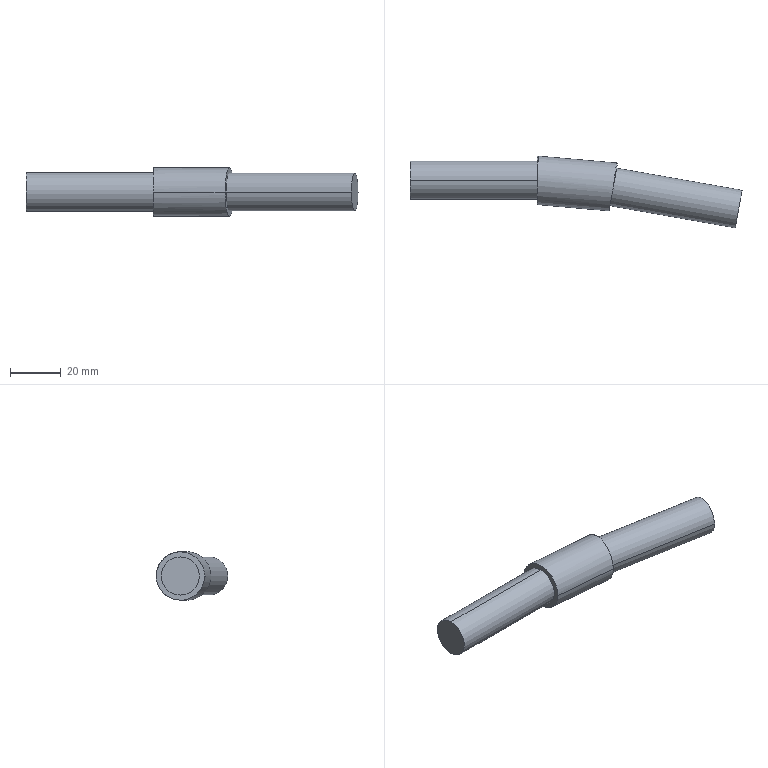Part | SolidWorks | features ICE 2, Sweep 1 | 1 solid | 13 faces | box 130.429 x 28.183 x 19 mm | volume 26177 mm3 | cylinder 9 | plane 4 | commonest cylinder face diameters 19 x5 15 x4
STEP:
#1=CARTESIAN_POINT('',(81.188,4.771,0.));
#2=VERTEX_POINT('',#1);
#3=CARTESIAN_POINT('',(78.583,-10.001,0.));
#4=VERTEX_POINT('',#3);
#5=CARTESIAN_POINT('',(79.886,-2.615,0.));
#6=DIRECTION('',(0.9848,-0.1736,0.));
#7=DIRECTION('',(0.1736,0.9848,0.));
#8=AXIS2_PLACEMENT_3D('',#5,#6,#7);
#9=CIRCLE('',#8,7.5);
#10=EDGE_CURVE('',#2,#4,#9,.T.);
#11=ORIENTED_EDGE('',*,*,#10,.T.);
#12=CARTESIAN_POINT('',(127.824,-18.683,0.));
#13=VERTEX_POINT('',#12);
#14=CARTESIAN_POINT('',(78.583,-10.001,0.));
#15=DIRECTION('',(0.9848,-0.1736,0.));
#16=VECTOR('',#15,1000.);
#17=LINE('',#14,#16);
#18=EDGE_CURVE('',#4,#13,#17,.T.);
#19=ORIENTED_EDGE('',*,*,#18,.T.);
#20=CARTESIAN_POINT('',(130.429,-3.911,0.));
#21=VERTEX_POINT('',#20);
#22=CARTESIAN_POINT('',(129.126,-11.297,0.));
#23=DIRECTION('',(0.9848,-0.1736,0.));
#24=DIRECTION('',(0.1736,0.9848,0.));
#25=AXIS2_PLACEMENT_3D('',#22,#23,#24);
#26=CIRCLE('',#25,7.5);
#27=EDGE_CURVE('',#21,#13,#26,.T.);
#28=ORIENTED_EDGE('',*,*,#27,.F.);
#29=CARTESIAN_POINT('',(81.188,4.771,0.));
#30=DIRECTION('',(0.9848,-0.1736,0.));
#31=VECTOR('',#30,1000.);
#32=LINE('',#29,#31);
#33=EDGE_CURVE('',#2,#21,#32,.T.);
#34=ORIENTED_EDGE('',*,*,#33,.F.);
#35=EDGE_LOOP('',(#11,#19,#28,#34));
#36=FACE_OUTER_BOUND('',#35,.T.);
#37=CARTESIAN_POINT('',(79.886,-2.615,0.));
#38=DIRECTION('',(0.9848,-0.1736,0.));
#39=DIRECTION('',(0.1736,0.9848,0.));
#40=AXIS2_PLACEMENT_3D('',#37,#38,#39);
#41=CYLINDRICAL_SURFACE('',#40,7.5);
#42=ADVANCED_FACE('',(#36),#41,.T.);
#43=CARTESIAN_POINT('',(50.,0.,7.5));
#44=VERTEX_POINT('',#43);
#45=CARTESIAN_POINT('',(50.,0.,-7.5));
#46=VERTEX_POINT('',#45);
#47=CARTESIAN_POINT('',(50.,0.,0.));
#48=DIRECTION('',(-1.,0.,0.));
#49=DIRECTION('',(0.,0.,1.));
#50=AXIS2_PLACEMENT_3D('',#47,#48,#49);
#51=CIRCLE('',#50,7.5);
#52=EDGE_CURVE('',#44,#46,#51,.T.);
#53=ORIENTED_EDGE('',*,*,#52,.T.);
#54=CARTESIAN_POINT('',(0.,0.,-7.5));
#55=VERTEX_POINT('',#54);
#56=CARTESIAN_POINT('',(50.,0.,-7.5));
#57=DIRECTION('',(-1.,0.,0.));
#58=VECTOR('',#57,1000.);
#59=LINE('',#56,#58);
#60=EDGE_CURVE('',#46,#55,#59,.T.);
#61=ORIENTED_EDGE('',*,*,#60,.T.);
#62=CARTESIAN_POINT('',(0.,0.,7.5));
#63=VERTEX_POINT('',#62);
#64=CARTESIAN_POINT('',(0.,0.,0.));
#65=DIRECTION('',(-1.,0.,0.));
#66=DIRECTION('',(0.,0.,1.));
#67=AXIS2_PLACEMENT_3D('',#64,#65,#66);
#68=CIRCLE('',#67,7.5);
#69=EDGE_CURVE('',#63,#55,#68,.T.);
#70=ORIENTED_EDGE('',*,*,#69,.F.);
#71=CARTESIAN_POINT('',(50.,0.,7.5));
#72=DIRECTION('',(-1.,0.,0.));
#73=VECTOR('',#72,1000.);
#74=LINE('',#71,#73);
#75=EDGE_CURVE('',#44,#63,#74,.T.);
#76=ORIENTED_EDGE('',*,*,#75,.F.);
#77=EDGE_LOOP('',(#53,#61,#70,#76));
#78=FACE_OUTER_BOUND('',#77,.T.);
#79=CARTESIAN_POINT('',(50.,0.,0.));
#80=DIRECTION('',(-1.,0.,0.));
#81=DIRECTION('',(0.,0.,1.));
#82=AXIS2_PLACEMENT_3D('',#79,#80,#81);
#83=CYLINDRICAL_SURFACE('',#82,7.5);
#84=ADVANCED_FACE('',(#78),#83,.T.);
#85=CARTESIAN_POINT('',(81.127,6.813,0.));
#86=VERTEX_POINT('',#85);
#87=CARTESIAN_POINT('',(79.886,-2.615,-9.5));
#88=VERTEX_POINT('',#87);
#89=CARTESIAN_POINT('',(81.127,6.813,0.));
#90=CARTESIAN_POINT('',(81.127,6.813,-5.565));
#91=CARTESIAN_POINT('',(80.613,2.908,-9.5));
#92=CARTESIAN_POINT('',(79.886,-2.615,-9.5));
#93=(BOUNDED_CURVE()B_SPLINE_CURVE(3,(#89,#90,#91,#92),.UNSPECIFIED.,.F.,.T.)B_SPLINE_CURVE_WITH_KNOTS((4,4),(0.,1.571),.UNSPECIFIED.)CURVE()GEOMETRIC_REPRESENTATION_ITEM()RATIONAL_B_SPLINE_CURVE((1.,0.8047,0.8047,1.))REPRESENTATION_ITEM(''));
#94=EDGE_CURVE('',#86,#88,#93,.T.);
#95=ORIENTED_EDGE('',*,*,#94,.F.);
#96=CARTESIAN_POINT('',(81.535,6.741,0.));
#97=VERTEX_POINT('',#96);
#98=CARTESIAN_POINT('',(81.535,6.741,0.));
#99=DIRECTION('',(0.9848,-0.1736,0.));
#100=VECTOR('',#99,1000.);
#101=LINE('',#98,#100);
#102=EDGE_CURVE('',#86,#97,#101,.T.);
#103=ORIENTED_EDGE('',*,*,#102,.T.);
#104=CARTESIAN_POINT('',(79.886,-2.615,0.));
#105=DIRECTION('',(0.9848,-0.1736,0.));
#106=DIRECTION('',(0.1736,0.9848,0.));
#107=AXIS2_PLACEMENT_3D('',#104,#105,#106);
#108=CIRCLE('',#107,9.5);
#109=EDGE_CURVE('',#88,#97,#108,.T.);
#110=ORIENTED_EDGE('',*,*,#109,.F.);
#111=EDGE_LOOP('',(#95,#103,#110));
#112=FACE_OUTER_BOUND('',#111,.T.);
#113=CARTESIAN_POINT('',(79.886,-2.615,0.));
#114=DIRECTION('',(0.9848,-0.1736,0.));
#115=DIRECTION('',(0.1736,0.9848,0.));
#116=AXIS2_PLACEMENT_3D('',#113,#114,#115);
#117=CYLINDRICAL_SURFACE('',#116,9.5);
#118=ADVANCED_FACE('',(#112),#117,.T.);
#119=CARTESIAN_POINT('',(50.,0.,9.5));
#120=VERTEX_POINT('',#119);
#121=CARTESIAN_POINT('',(50.,-9.536,0.));
#122=VERTEX_POINT('',#121);
#123=CARTESIAN_POINT('',(50.,0.,9.5));
#124=CARTESIAN_POINT('',(50.,-5.586,9.5));
#125=CARTESIAN_POINT('',(50.,-9.536,5.565));
#126=CARTESIAN_POINT('',(50.,-9.536,0.));
#127=(BOUNDED_CURVE()B_SPLINE_CURVE(3,(#123,#124,#125,#126),.UNSPECIFIED.,.F.,.T.)B_SPLINE_CURVE_WITH_KNOTS((4,4),(4.712,6.283),.UNSPECIFIED.)CURVE()GEOMETRIC_REPRESENTATION_ITEM()RATIONAL_B_SPLINE_CURVE((1.,0.8047,0.8047,1.))REPRESENTATION_ITEM(''));
#128=EDGE_CURVE('',#120,#122,#127,.T.);
#129=ORIENTED_EDGE('',*,*,#128,.T.);
#130=CARTESIAN_POINT('',(78.23,-12.006,0.));
#131=VERTEX_POINT('',#130);
#132=CARTESIAN_POINT('',(49.172,-9.464,0.));
#133=DIRECTION('',(0.9962,-0.08716,0.));
#134=VECTOR('',#133,1000.);
#135=LINE('',#132,#134);
#136=EDGE_CURVE('',#122,#131,#135,.T.);
#137=ORIENTED_EDGE('',*,*,#136,.T.);
#138=CARTESIAN_POINT('',(79.886,-2.615,9.5));
#139=VERTEX_POINT('',#138);
#140=CARTESIAN_POINT('',(78.23,-12.006,0.));
#141=CARTESIAN_POINT('',(78.23,-12.006,5.565));
#142=CARTESIAN_POINT('',(78.916,-8.116,9.5));
#143=CARTESIAN_POINT('',(79.886,-2.615,9.5));
#144=(BOUNDED_CURVE()B_SPLINE_CURVE(3,(#140,#141,#142,#143),.UNSPECIFIED.,.F.,.T.)B_SPLINE_CURVE_WITH_KNOTS((4,4),(3.142,4.712),.UNSPECIFIED.)CURVE()GEOMETRIC_REPRESENTATION_ITEM()RATIONAL_B_SPLINE_CURVE((1.,0.8047,0.8047,1.))REPRESENTATION_ITEM(''));
#145=EDGE_CURVE('',#131,#139,#144,.T.);
#146=ORIENTED_EDGE('',*,*,#145,.T.);
#147=CARTESIAN_POINT('',(79.886,-2.615,9.5));
#148=CARTESIAN_POINT('',(80.613,2.908,9.5));
#149=CARTESIAN_POINT('',(81.127,6.813,5.565));
#150=CARTESIAN_POINT('',(81.127,6.813,0.));
#151=(BOUNDED_CURVE()B_SPLINE_CURVE(3,(#147,#148,#149,#150),.UNSPECIFIED.,.F.,.T.)B_SPLINE_CURVE_WITH_KNOTS((4,4),(4.712,6.283),.UNSPECIFIED.)CURVE()GEOMETRIC_REPRESENTATION_ITEM()RATIONAL_B_SPLINE_CURVE((1.,0.8047,0.8047,1.))REPRESENTATION_ITEM(''));
#152=EDGE_CURVE('',#139,#86,#151,.T.);
#153=ORIENTED_EDGE('',*,*,#152,.T.);
#154=CARTESIAN_POINT('',(50.415,9.5,0.));
#155=VERTEX_POINT('',#154);
#156=CARTESIAN_POINT('',(50.828,9.464,0.));
#157=DIRECTION('',(0.9962,-0.08716,0.));
#158=VECTOR('',#157,1000.);
#159=LINE('',#156,#158);
#160=EDGE_CURVE('',#155,#86,#159,.T.);
#161=ORIENTED_EDGE('',*,*,#160,.F.);
#162=CARTESIAN_POINT('',(50.415,9.5,0.));
#163=CARTESIAN_POINT('',(50.415,9.5,5.565));
#164=CARTESIAN_POINT('',(50.243,5.565,9.5));
#165=CARTESIAN_POINT('',(50.,0.,9.5));
#166=(BOUNDED_CURVE()B_SPLINE_CURVE(3,(#162,#163,#164,#165),.UNSPECIFIED.,.F.,.T.)B_SPLINE_CURVE_WITH_KNOTS((4,4),(3.142,4.712),.UNSPECIFIED.)CURVE()GEOMETRIC_REPRESENTATION_ITEM()RATIONAL_B_SPLINE_CURVE((1.,0.8047,0.8047,1.))REPRESENTATION_ITEM(''));
#167=EDGE_CURVE('',#155,#120,#166,.T.);
#168=ORIENTED_EDGE('',*,*,#167,.T.);
#169=EDGE_LOOP('',(#129,#137,#146,#153,#161,#168));
#170=FACE_OUTER_BOUND('',#169,.T.);
#171=CARTESIAN_POINT('',(50.,0.,0.));
#172=DIRECTION('',(0.9962,-0.08716,0.));
#173=DIRECTION('',(0.08716,0.9962,0.));
#174=AXIS2_PLACEMENT_3D('',#171,#172,#173);
#175=CYLINDRICAL_SURFACE('',#174,9.5);
#176=ADVANCED_FACE('',(#170),#175,.T.);
#177=ORIENTED_EDGE('',*,*,#136,.F.);
#178=CARTESIAN_POINT('',(50.,0.,-9.5));
#179=VERTEX_POINT('',#178);
#180=CARTESIAN_POINT('',(50.,-9.536,0.));
#181=CARTESIAN_POINT('',(50.,-9.536,-5.565));
#182=CARTESIAN_POINT('',(50.,-5.586,-9.5));
#183=CARTESIAN_POINT('',(50.,0.,-9.5));
#184=(BOUNDED_CURVE()B_SPLINE_CURVE(3,(#180,#181,#182,#183),.UNSPECIFIED.,.F.,.T.)B_SPLINE_CURVE_WITH_KNOTS((4,4),(0.,1.571),.UNSPECIFIED.)CURVE()GEOMETRIC_REPRESENTATION_ITEM()RATIONAL_B_SPLINE_CURVE((1.,0.8047,0.8047,1.))REPRESENTATION_ITEM(''));
#185=EDGE_CURVE('',#122,#179,#184,.T.);
#186=ORIENTED_EDGE('',*,*,#185,.T.);
#187=CARTESIAN_POINT('',(50.,0.,-9.5));
#188=CARTESIAN_POINT('',(50.243,5.565,-9.5));
#189=CARTESIAN_POINT('',(50.415,9.5,-5.565));
#190=CARTESIAN_POINT('',(50.415,9.5,0.));
#191=(BOUNDED_CURVE()B_SPLINE_CURVE(3,(#187,#188,#189,#190),.UNSPECIFIED.,.F.,.T.)B_SPLINE_CURVE_WITH_KNOTS((4,4),(1.571,3.142),.UNSPECIFIED.)CURVE()GEOMETRIC_REPRESENTATION_ITEM()RATIONAL_B_SPLINE_CURVE((1.,0.8047,0.8047,1.))REPRESENTATION_ITEM(''));
#192=EDGE_CURVE('',#179,#155,#191,.T.);
#193=ORIENTED_EDGE('',*,*,#192,.T.);
#194=ORIENTED_EDGE('',*,*,#160,.T.);
#195=ORIENTED_EDGE('',*,*,#94,.T.);
#196=CARTESIAN_POINT('',(79.886,-2.615,-9.5));
#197=CARTESIAN_POINT('',(78.916,-8.116,-9.5));
#198=CARTESIAN_POINT('',(78.23,-12.006,-5.565));
#199=CARTESIAN_POINT('',(78.23,-12.006,0.));
#200=(BOUNDED_CURVE()B_SPLINE_CURVE(3,(#196,#197,#198,#199),.UNSPECIFIED.,.F.,.T.)B_SPLINE_CURVE_WITH_KNOTS((4,4),(1.571,3.142),.UNSPECIFIED.)CURVE()GEOMETRIC_REPRESENTATION_ITEM()RATIONAL_B_SPLINE_CURVE((1.,0.8047,0.8047,1.))REPRESENTATION_ITEM(''));
#201=EDGE_CURVE('',#88,#131,#200,.T.);
#202=ORIENTED_EDGE('',*,*,#201,.T.);
#203=EDGE_LOOP('',(#177,#186,#193,#194,#195,#202));
#204=FACE_OUTER_BOUND('',#203,.T.);
#205=CARTESIAN_POINT('',(50.,0.,0.));
#206=DIRECTION('',(0.9962,-0.08716,0.));
#207=DIRECTION('',(0.08716,0.9962,0.));
#208=AXIS2_PLACEMENT_3D('',#205,#206,#207);
#209=CYLINDRICAL_SURFACE('',#208,9.5);
#210=ADVANCED_FACE('',(#204),#209,.T.);
#211=ORIENTED_EDGE('',*,*,#102,.F.);
#212=ORIENTED_EDGE('',*,*,#152,.F.);
#213=CARTESIAN_POINT('',(79.886,-2.615,0.));
#214=DIRECTION('',(0.9848,-0.1736,0.));
#215=DIRECTION('',(0.1736,0.9848,0.));
#216=AXIS2_PLACEMENT_3D('',#213,#214,#215);
#217=CIRCLE('',#216,9.5);
#218=EDGE_CURVE('',#97,#139,#217,.T.);
#219=ORIENTED_EDGE('',*,*,#218,.F.);
#220=EDGE_LOOP('',(#211,#212,#219));
#221=FACE_OUTER_BOUND('',#220,.T.);
#222=CARTESIAN_POINT('',(79.886,-2.615,0.));
#223=DIRECTION('',(0.9848,-0.1736,0.));
#224=DIRECTION('',(0.1736,0.9848,0.));
#225=AXIS2_PLACEMENT_3D('',#222,#223,#224);
#226=CYLINDRICAL_SURFACE('',#225,9.5);
#227=ADVANCED_FACE('',(#221),#226,.T.);
#228=CARTESIAN_POINT('',(50.,0.,0.));
#229=DIRECTION('',(-1.,0.,0.));
#230=DIRECTION('',(0.,0.,1.));
#231=AXIS2_PLACEMENT_3D('',#228,#229,#230);
#232=CIRCLE('',#231,9.5);
#233=EDGE_CURVE('',#120,#179,#232,.T.);
#234=ORIENTED_EDGE('',*,*,#233,.F.);
#235=ORIENTED_EDGE('',*,*,#167,.F.);
#236=ORIENTED_EDGE('',*,*,#192,.F.);
#237=EDGE_LOOP('',(#234,#235,#236));
#238=FACE_OUTER_BOUND('',#237,.T.);
#239=CARTESIAN_POINT('',(76.87,0.,0.));
#240=DIRECTION('',(-1.,0.,0.));
#241=DIRECTION('',(0.,0.,1.));
#242=AXIS2_PLACEMENT_3D('',#239,#240,#241);
#243=CYLINDRICAL_SURFACE('',#242,9.5);
#244=ADVANCED_FACE('',(#238),#243,.T.);
#245=ORIENTED_EDGE('',*,*,#233,.T.);
#246=ORIENTED_EDGE('',*,*,#185,.F.);
#247=ORIENTED_EDGE('',*,*,#128,.F.);
#248=EDGE_LOOP('',(#245,#246,#247));
#249=FACE_OUTER_BOUND('',#248,.T.);
#250=ORIENTED_EDGE('',*,*,#52,.F.);
#251=CARTESIAN_POINT('',(50.,0.,0.));
#252=DIRECTION('',(-1.,0.,0.));
#253=DIRECTION('',(0.,0.,1.));
#254=AXIS2_PLACEMENT_3D('',#251,#252,#253);
#255=CIRCLE('',#254,7.5);
#256=EDGE_CURVE('',#46,#44,#255,.T.);
#257=ORIENTED_EDGE('',*,*,#256,.F.);
#258=EDGE_LOOP('',(#250,#257));
#259=FACE_BOUND('',#258,.T.);
#260=CARTESIAN_POINT('',(50.,-5.576,0.));
#261=DIRECTION('',(-1.,0.,0.));
#262=DIRECTION('',(0.,0.,1.));
#263=AXIS2_PLACEMENT_3D('',#260,#261,#262);
#264=PLANE('',#263);
#265=ADVANCED_FACE('',(#249,#259),#264,.T.);
#266=ORIENTED_EDGE('',*,*,#60,.F.);
#267=ORIENTED_EDGE('',*,*,#256,.T.);
#268=ORIENTED_EDGE('',*,*,#75,.T.);
#269=CARTESIAN_POINT('',(0.,0.,0.));
#270=DIRECTION('',(-1.,0.,0.));
#271=DIRECTION('',(0.,0.,1.));
#272=AXIS2_PLACEMENT_3D('',#269,#270,#271);
#273=CIRCLE('',#272,7.5);
#274=EDGE_CURVE('',#55,#63,#273,.T.);
#275=ORIENTED_EDGE('',*,*,#274,.F.);
#276=EDGE_LOOP('',(#266,#267,#268,#275));
#277=FACE_OUTER_BOUND('',#276,.T.);
#278=CARTESIAN_POINT('',(50.,0.,0.));
#279=DIRECTION('',(-1.,0.,0.));
#280=DIRECTION('',(0.,0.,1.));
#281=AXIS2_PLACEMENT_3D('',#278,#279,#280);
#282=CYLINDRICAL_SURFACE('',#281,7.5);
#283=ADVANCED_FACE('',(#277),#282,.T.);
#284=ORIENTED_EDGE('',*,*,#69,.T.);
#285=ORIENTED_EDGE('',*,*,#274,.T.);
#286=EDGE_LOOP('',(#284,#285));
#287=FACE_OUTER_BOUND('',#286,.T.);
#288=CARTESIAN_POINT('',(0.,0.,0.));
#289=DIRECTION('',(1.,0.,0.));
#290=DIRECTION('',(0.,0.,-1.));
#291=AXIS2_PLACEMENT_3D('',#288,#289,#290);
#292=PLANE('',#291);
#293=ADVANCED_FACE('',(#287),#292,.F.);
#294=ORIENTED_EDGE('',*,*,#109,.T.);
#295=ORIENTED_EDGE('',*,*,#218,.T.);
#296=ORIENTED_EDGE('',*,*,#145,.F.);
#297=ORIENTED_EDGE('',*,*,#201,.F.);
#298=EDGE_LOOP('',(#294,#295,#296,#297));
#299=FACE_OUTER_BOUND('',#298,.T.);
#300=ORIENTED_EDGE('',*,*,#10,.F.);
#301=CARTESIAN_POINT('',(79.886,-2.615,0.));
#302=DIRECTION('',(0.9848,-0.1736,0.));
#303=DIRECTION('',(0.1736,0.9848,0.));
#304=AXIS2_PLACEMENT_3D('',#301,#302,#303);
#305=CIRCLE('',#304,7.5);
#306=EDGE_CURVE('',#4,#2,#305,.T.);
#307=ORIENTED_EDGE('',*,*,#306,.F.);
#308=EDGE_LOOP('',(#300,#307));
#309=FACE_BOUND('',#308,.T.);
#310=CARTESIAN_POINT('',(78.942,-7.966,0.));
#311=DIRECTION('',(0.9848,-0.1736,0.));
#312=DIRECTION('',(0.1736,0.9848,0.));
#313=AXIS2_PLACEMENT_3D('',#310,#311,#312);
#314=PLANE('',#313);
#315=ADVANCED_FACE('',(#299,#309),#314,.T.);
#316=ORIENTED_EDGE('',*,*,#18,.F.);
#317=ORIENTED_EDGE('',*,*,#306,.T.);
#318=ORIENTED_EDGE('',*,*,#33,.T.);
#319=CARTESIAN_POINT('',(129.126,-11.297,0.));
#320=DIRECTION('',(0.9848,-0.1736,0.));
#321=DIRECTION('',(0.1736,0.9848,0.));
#322=AXIS2_PLACEMENT_3D('',#319,#320,#321);
#323=CIRCLE('',#322,7.5);
#324=EDGE_CURVE('',#13,#21,#323,.T.);
#325=ORIENTED_EDGE('',*,*,#324,.F.);
#326=EDGE_LOOP('',(#316,#317,#318,#325));
#327=FACE_OUTER_BOUND('',#326,.T.);
#328=CARTESIAN_POINT('',(79.886,-2.615,0.));
#329=DIRECTION('',(0.9848,-0.1736,0.));
#330=DIRECTION('',(0.1736,0.9848,0.));
#331=AXIS2_PLACEMENT_3D('',#328,#329,#330);
#332=CYLINDRICAL_SURFACE('',#331,7.5);
#333=ADVANCED_FACE('',(#327),#332,.T.);
#334=ORIENTED_EDGE('',*,*,#27,.T.);
#335=ORIENTED_EDGE('',*,*,#324,.T.);
#336=EDGE_LOOP('',(#334,#335));
#337=FACE_OUTER_BOUND('',#336,.T.);
#338=CARTESIAN_POINT('',(129.126,-11.297,0.));
#339=DIRECTION('',(0.9848,-0.1736,0.));
#340=DIRECTION('',(0.1736,0.9848,0.));
#341=AXIS2_PLACEMENT_3D('',#338,#339,#340);
#342=PLANE('',#341);
#343=ADVANCED_FACE('',(#337),#342,.T.);
#344=CLOSED_SHELL('',(#42,#84,#118,#176,#210,#227,#244,#265,#283,#293,#315,#333,#343));
#345=MANIFOLD_SOLID_BREP('',#344);
#346=CARTESIAN_POINT('',(0.,0.,0.));
#347=DIRECTION('',(0.,0.,1.));
#348=DIRECTION('',(1.,0.,0.));
#349=AXIS2_PLACEMENT_3D('',#346,#347,#348);
#350=(LENGTH_UNIT()NAMED_UNIT(*)SI_UNIT(.MILLI.,.METRE.));
#351=UNCERTAINTY_MEASURE_WITH_UNIT(LENGTH_MEASURE(0.00001),#350,'','');
#352=(NAMED_UNIT(*)PLANE_ANGLE_UNIT()SI_UNIT($,.RADIAN.));
#353=(NAMED_UNIT(*)SI_UNIT($,.STERADIAN.)SOLID_ANGLE_UNIT());
#354=(GEOMETRIC_REPRESENTATION_CONTEXT(3)GLOBAL_UNCERTAINTY_ASSIGNED_CONTEXT((#351))GLOBAL_UNIT_ASSIGNED_CONTEXT((#350,#352,#353))REPRESENTATION_CONTEXT('',''));
#355=ADVANCED_BREP_SHAPE_REPRESENTATION('',(#345,#349),#354);